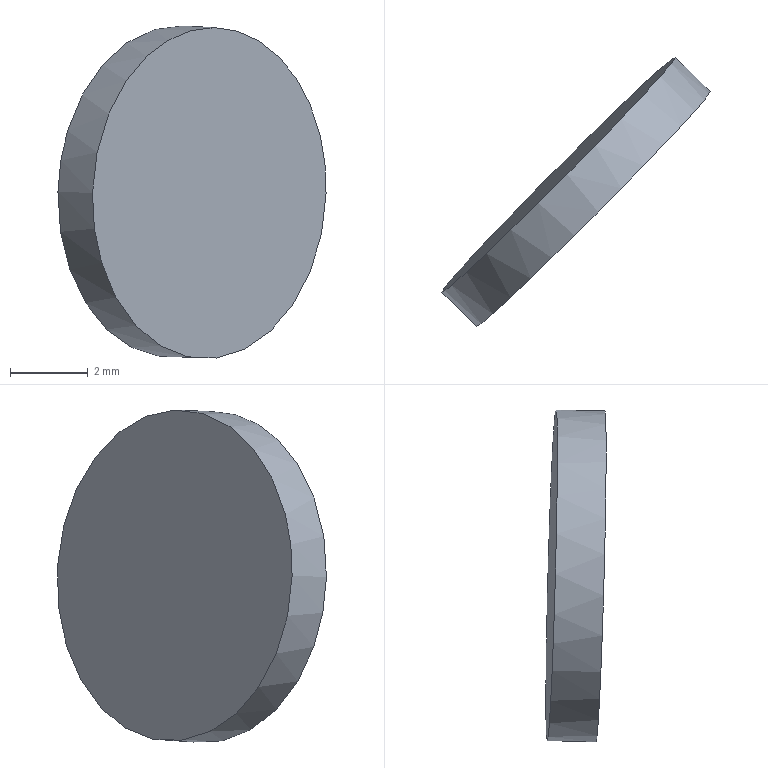Part | STEP file | gslz 2016.10.28-13_id1114_x_t | 1 solid | 3 faces | box 6.882 x 6.913 x 8.538 mm | volume 70.931 mm3 | spline 2 | cylinder 1 | commonest cylinder face diameters 8.5 x1
STEP:
#1=CARTESIAN_POINT('',(0.,0.,0.));
#2=DIRECTION('',(0.,0.,1.));
#3=DIRECTION('',(1.,0.,0.));
#4=AXIS2_PLACEMENT_3D('',#1,#2,#3);
#5=CARTESIAN_POINT('',(428.577,221.709,-30.621));
#6=VERTEX_POINT('',#5);
#7=CARTESIAN_POINT('',(428.577,221.709,-30.621));
#8=CARTESIAN_POINT('',(428.565,221.72,-31.097));
#9=CARTESIAN_POINT('',(428.611,221.79,-31.579));
#10=CARTESIAN_POINT('',(428.711,221.913,-32.027));
#11=CARTESIAN_POINT('',(428.811,222.036,-32.476));
#12=CARTESIAN_POINT('',(428.967,222.214,-32.903));
#13=CARTESIAN_POINT('',(429.168,222.434,-33.275));
#14=CARTESIAN_POINT('',(429.368,222.654,-33.646));
#15=CARTESIAN_POINT('',(429.618,222.921,-33.971));
#16=CARTESIAN_POINT('',(429.896,223.213,-34.223));
#17=CARTESIAN_POINT('',(430.174,223.506,-34.475));
#18=CARTESIAN_POINT('',(430.488,223.831,-34.661));
#19=CARTESIAN_POINT('',(430.813,224.163,-34.765));
#20=CARTESIAN_POINT('',(431.137,224.495,-34.869));
#21=CARTESIAN_POINT('',(431.481,224.842,-34.895));
#22=CARTESIAN_POINT('',(431.815,225.175,-34.84));
#23=CARTESIAN_POINT('',(432.15,225.509,-34.785));
#24=CARTESIAN_POINT('',(432.484,225.839,-34.648));
#25=CARTESIAN_POINT('',(432.791,226.137,-34.44));
#26=CARTESIAN_POINT('',(433.097,226.435,-34.231));
#27=CARTESIAN_POINT('',(433.385,226.71,-33.946));
#28=CARTESIAN_POINT('',(433.629,226.939,-33.608));
#29=CARTESIAN_POINT('',(433.873,227.168,-33.271));
#30=CARTESIAN_POINT('',(434.081,227.357,-32.87));
#31=CARTESIAN_POINT('',(434.235,227.491,-32.441));
#32=CARTESIAN_POINT('',(434.389,227.625,-32.011));
#33=CARTESIAN_POINT('',(434.494,227.708,-31.54));
#34=CARTESIAN_POINT('',(434.541,227.732,-31.068));
#35=CARTESIAN_POINT('',(434.588,227.755,-30.595));
#36=CARTESIAN_POINT('',(434.578,227.721,-30.107));
#37=CARTESIAN_POINT('',(434.512,227.633,-29.644));
#38=CARTESIAN_POINT('',(434.447,227.544,-29.182));
#39=CARTESIAN_POINT('',(434.323,227.397,-28.732));
#40=CARTESIAN_POINT('',(434.152,227.205,-28.331));
#41=CARTESIAN_POINT('',(433.981,227.014,-27.931));
#42=CARTESIAN_POINT('',(433.758,226.771,-27.569));
#43=CARTESIAN_POINT('',(433.502,226.498,-27.276));
#44=CARTESIAN_POINT('',(433.245,226.226,-26.983));
#45=CARTESIAN_POINT('',(432.947,225.915,-26.751));
#46=CARTESIAN_POINT('',(432.633,225.591,-26.598));
#47=CARTESIAN_POINT('',(432.319,225.268,-26.446));
#48=CARTESIAN_POINT('',(431.981,224.924,-26.369));
#49=CARTESIAN_POINT('',(431.645,224.586,-26.374));
#50=CARTESIAN_POINT('',(431.31,224.249,-26.379));
#51=CARTESIAN_POINT('',(430.968,223.91,-26.467));
#52=CARTESIAN_POINT('',(430.649,223.597,-26.629));
#53=CARTESIAN_POINT('',(430.33,223.284,-26.791));
#54=CARTESIAN_POINT('',(430.024,222.988,-27.032));
#55=CARTESIAN_POINT('',(429.757,222.734,-27.333));
#56=CARTESIAN_POINT('',(429.49,222.48,-27.634));
#57=CARTESIAN_POINT('',(429.254,222.261,-28.003));
#58=CARTESIAN_POINT('',(429.07,222.096,-28.409));
#59=CARTESIAN_POINT('',(428.885,221.93,-28.815));
#60=CARTESIAN_POINT('',(428.746,221.813,-29.269));
#61=CARTESIAN_POINT('',(428.665,221.753,-29.734));
#62=CARTESIAN_POINT('',(428.614,221.716,-30.025));
#63=CARTESIAN_POINT('',(428.584,221.701,-30.324));
#64=CARTESIAN_POINT('',(428.577,221.709,-30.621));
#65=B_SPLINE_CURVE_WITH_KNOTS('',3,(#7,#8,#9,#10,#11,#12,#13,#14,#15,#16,#17,#18,#19,#20,#21,#22,#23,#24,#25,#26,#27,#28,#29,#30,#31,#32,#33,#34,#35,#36,#37,#38,#39,#40,#41,#42,#43,#44,#45,#46,#47,#48,#49,#50,#51,#52,#53,#54,#55,#56,#57,#58,#59,#60,#61,#62,#63,#64),.UNSPECIFIED.,.T.,.F.,(1,3,3,3,3,3,3,3,3,3,3,3,3,3,3,3,3,3,3,3,3,1),(-0.03332,0.,0.0537,0.1074,0.1611,0.2148,0.2685,0.3222,0.3759,0.4296,0.4833,0.537,0.5907,0.6445,0.6982,0.7519,0.8056,0.8593,0.913,0.9667,1.,1.054),.UNSPECIFIED.);
#66=CARTESIAN_POINT('',(417.862,211.656,-45.368));
#67=CARTESIAN_POINT('',(417.657,211.178,-39.851));
#68=CARTESIAN_POINT('',(417.452,210.7,-34.333));
#69=CARTESIAN_POINT('',(417.248,210.222,-28.816));
#70=CARTESIAN_POINT('',(417.043,209.744,-23.299));
#71=CARTESIAN_POINT('',(416.839,209.265,-17.782));
#72=CARTESIAN_POINT('',(423.082,216.876,-44.722));
#73=CARTESIAN_POINT('',(422.877,216.398,-39.205));
#74=CARTESIAN_POINT('',(422.673,215.92,-33.688));
#75=CARTESIAN_POINT('',(422.468,215.442,-28.17));
#76=CARTESIAN_POINT('',(422.264,214.964,-22.653));
#77=CARTESIAN_POINT('',(422.059,214.486,-17.136));
#78=CARTESIAN_POINT('',(428.302,222.096,-44.076));
#79=CARTESIAN_POINT('',(428.098,221.618,-38.559));
#80=CARTESIAN_POINT('',(427.893,221.14,-33.042));
#81=CARTESIAN_POINT('',(427.688,220.662,-27.524));
#82=CARTESIAN_POINT('',(427.484,220.184,-22.007));
#83=CARTESIAN_POINT('',(427.279,219.706,-16.49));
#84=CARTESIAN_POINT('',(433.522,227.317,-43.43));
#85=CARTESIAN_POINT('',(433.318,226.839,-37.913));
#86=CARTESIAN_POINT('',(433.113,226.361,-32.396));
#87=CARTESIAN_POINT('',(432.909,225.882,-26.879));
#88=CARTESIAN_POINT('',(432.704,225.404,-21.361));
#89=CARTESIAN_POINT('',(432.5,224.926,-15.844));
#90=CARTESIAN_POINT('',(438.743,232.537,-42.784));
#91=CARTESIAN_POINT('',(438.538,232.059,-37.267));
#92=CARTESIAN_POINT('',(438.334,231.581,-31.75));
#93=CARTESIAN_POINT('',(438.129,231.103,-26.233));
#94=CARTESIAN_POINT('',(437.924,230.625,-20.715));
#95=CARTESIAN_POINT('',(437.72,230.147,-15.198));
#96=CARTESIAN_POINT('',(443.963,237.757,-42.139));
#97=CARTESIAN_POINT('',(443.758,237.279,-36.621));
#98=CARTESIAN_POINT('',(443.554,236.801,-31.104));
#99=CARTESIAN_POINT('',(443.349,236.323,-25.587));
#100=CARTESIAN_POINT('',(443.145,235.845,-20.07));
#101=CARTESIAN_POINT('',(442.94,235.367,-14.552));
#102=B_SPLINE_SURFACE_WITH_KNOTS('',5,5,((#66,#67,#68,#69,#70,#71),(#72,#73,#74,#75,#76,#77),(#78,#79,#80,#81,#82,#83),(#84,#85,#86,#87,#88,#89),(#90,#91,#92,#93,#94,#95),(#96,#97,#98,#99,#100,#101)),.UNSPECIFIED.,.F.,.F.,.F.,(6,6),(6,6),(0.,1.),(0.,1.),.PIECEWISE_BEZIER_KNOTS.);
#103=CARTESIAN_POINT('',(0.4295,0.4843));
#104=CARTESIAN_POINT('',(0.4293,0.4807));
#105=CARTESIAN_POINT('',(0.429,0.4734));
#106=CARTESIAN_POINT('',(0.4291,0.4624));
#107=CARTESIAN_POINT('',(0.4299,0.4515));
#108=CARTESIAN_POINT('',(0.4312,0.4406));
#109=CARTESIAN_POINT('',(0.4331,0.43));
#110=CARTESIAN_POINT('',(0.4356,0.4196));
#111=CARTESIAN_POINT('',(0.4386,0.4094));
#112=CARTESIAN_POINT('',(0.4421,0.3995));
#113=CARTESIAN_POINT('',(0.4462,0.39));
#114=CARTESIAN_POINT('',(0.4508,0.3809));
#115=CARTESIAN_POINT('',(0.4558,0.3723));
#116=CARTESIAN_POINT('',(0.4613,0.3641));
#117=CARTESIAN_POINT('',(0.4672,0.3565));
#118=CARTESIAN_POINT('',(0.4735,0.3495));
#119=CARTESIAN_POINT('',(0.4801,0.3431));
#120=CARTESIAN_POINT('',(0.4871,0.3374));
#121=CARTESIAN_POINT('',(0.4944,0.3323));
#122=CARTESIAN_POINT('',(0.5019,0.328));
#123=CARTESIAN_POINT('',(0.5096,0.3243));
#124=CARTESIAN_POINT('',(0.5175,0.3215));
#125=CARTESIAN_POINT('',(0.5256,0.3194));
#126=CARTESIAN_POINT('',(0.5337,0.318));
#127=CARTESIAN_POINT('',(0.5419,0.3174));
#128=CARTESIAN_POINT('',(0.5501,0.3176));
#129=CARTESIAN_POINT('',(0.5582,0.3186));
#130=CARTESIAN_POINT('',(0.5663,0.3204));
#131=CARTESIAN_POINT('',(0.5743,0.3229));
#132=CARTESIAN_POINT('',(0.5821,0.3262));
#133=CARTESIAN_POINT('',(0.5897,0.3302));
#134=CARTESIAN_POINT('',(0.5971,0.335));
#135=CARTESIAN_POINT('',(0.6042,0.3404));
#136=CARTESIAN_POINT('',(0.6111,0.3466));
#137=CARTESIAN_POINT('',(0.6175,0.3533));
#138=CARTESIAN_POINT('',(0.6236,0.3606));
#139=CARTESIAN_POINT('',(0.6293,0.3685));
#140=CARTESIAN_POINT('',(0.6345,0.3769));
#141=CARTESIAN_POINT('',(0.6393,0.3858));
#142=CARTESIAN_POINT('',(0.6436,0.3951));
#143=CARTESIAN_POINT('',(0.6474,0.4048));
#144=CARTESIAN_POINT('',(0.6506,0.4149));
#145=CARTESIAN_POINT('',(0.6533,0.4253));
#146=CARTESIAN_POINT('',(0.6555,0.4358));
#147=CARTESIAN_POINT('',(0.6571,0.4465));
#148=CARTESIAN_POINT('',(0.6581,0.4574));
#149=CARTESIAN_POINT('',(0.6585,0.4684));
#150=CARTESIAN_POINT('',(0.6584,0.4794));
#151=CARTESIAN_POINT('',(0.6576,0.4903));
#152=CARTESIAN_POINT('',(0.6563,0.501));
#153=CARTESIAN_POINT('',(0.6544,0.5117));
#154=CARTESIAN_POINT('',(0.652,0.5222));
#155=CARTESIAN_POINT('',(0.6489,0.5324));
#156=CARTESIAN_POINT('',(0.6454,0.5422));
#157=CARTESIAN_POINT('',(0.6414,0.5517));
#158=CARTESIAN_POINT('',(0.6368,0.5608));
#159=CARTESIAN_POINT('',(0.6317,0.5695));
#160=CARTESIAN_POINT('',(0.6263,0.5777));
#161=CARTESIAN_POINT('',(0.6204,0.5852));
#162=CARTESIAN_POINT('',(0.6141,0.5922));
#163=CARTESIAN_POINT('',(0.6074,0.5986));
#164=CARTESIAN_POINT('',(0.6004,0.6044));
#165=CARTESIAN_POINT('',(0.5932,0.6095));
#166=CARTESIAN_POINT('',(0.5857,0.6138));
#167=CARTESIAN_POINT('',(0.578,0.6174));
#168=CARTESIAN_POINT('',(0.57,0.6203));
#169=CARTESIAN_POINT('',(0.562,0.6225));
#170=CARTESIAN_POINT('',(0.5539,0.6238));
#171=CARTESIAN_POINT('',(0.5457,0.6244));
#172=CARTESIAN_POINT('',(0.5375,0.6242));
#173=CARTESIAN_POINT('',(0.5293,0.6232));
#174=CARTESIAN_POINT('',(0.5212,0.6214));
#175=CARTESIAN_POINT('',(0.5133,0.6189));
#176=CARTESIAN_POINT('',(0.5055,0.6156));
#177=CARTESIAN_POINT('',(0.4979,0.6116));
#178=CARTESIAN_POINT('',(0.4904,0.6069));
#179=CARTESIAN_POINT('',(0.4833,0.6014));
#180=CARTESIAN_POINT('',(0.4765,0.5954));
#181=CARTESIAN_POINT('',(0.4701,0.5886));
#182=CARTESIAN_POINT('',(0.464,0.5813));
#183=CARTESIAN_POINT('',(0.4583,0.5734));
#184=CARTESIAN_POINT('',(0.453,0.565));
#185=CARTESIAN_POINT('',(0.4483,0.5561));
#186=CARTESIAN_POINT('',(0.444,0.5468));
#187=CARTESIAN_POINT('',(0.4402,0.537));
#188=CARTESIAN_POINT('',(0.4369,0.527));
#189=CARTESIAN_POINT('',(0.4342,0.5167));
#190=CARTESIAN_POINT('',(0.432,0.506));
#191=CARTESIAN_POINT('',(0.4304,0.4952));
#192=CARTESIAN_POINT('',(0.4297,0.4879));
#193=CARTESIAN_POINT('',(0.4295,0.4843));
#194=B_SPLINE_CURVE_WITH_KNOTS('',3,(#103,#104,#105,#106,#107,#108,#109,#110,#111,#112,#113,#114,#115,#116,#117,#118,#119,#120,#121,#122,#123,#124,#125,#126,#127,#128,#129,#130,#131,#132,#133,#134,#135,#136,#137,#138,#139,#140,#141,#142,#143,#144,#145,#146,#147,#148,#149,#150,#151,#152,#153,#154,#155,#156,#157,#158,#159,#160,#161,#162,#163,#164,#165,#166,#167,#168,#169,#170,#171,#172,#173,#174,#175,#176,#177,#178,#179,#180,#181,#182,#183,#184,#185,#186,#187,#188,#189,#190,#191,#192,#193),.UNSPECIFIED.,.T.,.F.,(4,1,1,1,1,1,1,1,1,1,1,1,1,1,1,1,1,1,1,1,1,1,1,1,1,1,1,1,1,1,1,1,1,1,1,1,1,1,1,1,1,1,1,1,1,1,1,1,1,1,1,1,1,1,1,1,1,1,1,1,1,1,1,1,1,1,1,1,1,1,1,1,1,1,1,1,1,1,1,1,1,1,1,1,1,1,1,1,4),(0.,0.01136,0.02273,0.03409,0.04545,0.05682,0.06818,0.07955,0.09091,0.1023,0.1136,0.125,0.1364,0.1477,0.1591,0.1705,0.1818,0.1932,0.2045,0.2159,0.2273,0.2386,0.25,0.2614,0.2727,0.2841,0.2955,0.3068,0.3182,0.3295,0.3409,0.3523,0.3636,0.375,0.3864,0.3977,0.4091,0.4205,0.4318,0.4432,0.4545,0.4659,0.4773,0.4886,0.5,0.5114,0.5227,0.5341,0.5455,0.5568,0.5682,0.5795,0.5909,0.6023,0.6136,0.625,0.6364,0.6477,0.6591,0.6705,0.6818,0.6932,0.7045,0.7159,0.7273,0.7386,0.75,0.7614,0.7727,0.7841,0.7955,0.8068,0.8182,0.8295,0.8409,0.8523,0.8636,0.875,0.8864,0.8977,0.9091,0.9205,0.9318,0.9432,0.9545,0.9659,0.9773,0.9886,1.),.QUASI_UNIFORM_KNOTS.);
#195=(GEOMETRIC_REPRESENTATION_CONTEXT(2)PARAMETRIC_REPRESENTATION_CONTEXT()REPRESENTATION_CONTEXT('',''));
#196=DEFINITIONAL_REPRESENTATION('',(#194),#195);
#197=PCURVE('',#102,#196);
#198=CARTESIAN_POINT('',(433.912,222.398,-30.736));
#199=DIRECTION('',(-0.7088,0.7045,0.03477));
#200=DIRECTION('',(-0.705,-0.7093,0.));
#201=AXIS2_PLACEMENT_3D('',#198,#199,#200);
#202=CYLINDRICAL_SURFACE('',#201,4.25);
#203=CARTESIAN_POINT('',(6.283,3.3));
#204=CARTESIAN_POINT('',(0.,3.3));
#205=B_SPLINE_CURVE_WITH_KNOTS('',1,(#203,#204),.UNSPECIFIED.,.F.,.F.,(2,2),(0.,1.),.PIECEWISE_BEZIER_KNOTS.);
#206=(GEOMETRIC_REPRESENTATION_CONTEXT(2)PARAMETRIC_REPRESENTATION_CONTEXT()REPRESENTATION_CONTEXT('',''));
#207=DEFINITIONAL_REPRESENTATION('',(#205),#206);
#208=PCURVE('',#202,#207);
#209=SURFACE_CURVE('',#65,(#197,#208),.PCURVE_S1.);
#210=EDGE_CURVE('',#6,#6,#209,.T.);
#211=ORIENTED_EDGE('',*,*,#210,.T.);
#212=EDGE_LOOP('',(#211));
#213=FACE_BOUND('',#212,.F.);
#214=ADVANCED_FACE('',(#213),#102,.F.);
#215=CARTESIAN_POINT('',(435.455,226.857,-30.665));
#216=VERTEX_POINT('',#215);
#217=CARTESIAN_POINT('',(429.463,220.828,-30.665));
#218=VERTEX_POINT('',#217);
#219=CARTESIAN_POINT('',(435.455,226.857,-30.665));
#220=CARTESIAN_POINT('',(435.443,226.868,-31.14));
#221=CARTESIAN_POINT('',(435.373,226.822,-31.622));
#222=CARTESIAN_POINT('',(435.251,226.721,-32.071));
#223=CARTESIAN_POINT('',(435.129,226.621,-32.519));
#224=CARTESIAN_POINT('',(434.951,226.463,-32.947));
#225=CARTESIAN_POINT('',(434.733,226.261,-33.318));
#226=CARTESIAN_POINT('',(434.514,226.06,-33.689));
#227=CARTESIAN_POINT('',(434.249,225.808,-34.014));
#228=CARTESIAN_POINT('',(433.958,225.528,-34.266));
#229=CARTESIAN_POINT('',(433.667,225.249,-34.518));
#230=CARTESIAN_POINT('',(433.344,224.932,-34.704));
#231=CARTESIAN_POINT('',(433.014,224.606,-34.809));
#232=CARTESIAN_POINT('',(432.684,224.279,-34.913));
#233=CARTESIAN_POINT('',(432.339,223.933,-34.939));
#234=CARTESIAN_POINT('',(432.008,223.597,-34.884));
#235=CARTESIAN_POINT('',(431.676,223.26,-34.829));
#236=CARTESIAN_POINT('',(431.348,222.924,-34.691));
#237=CARTESIAN_POINT('',(431.052,222.616,-34.483));
#238=CARTESIAN_POINT('',(430.756,222.307,-34.275));
#239=CARTESIAN_POINT('',(430.483,222.018,-33.99));
#240=CARTESIAN_POINT('',(430.255,221.773,-33.652));
#241=CARTESIAN_POINT('',(430.028,221.527,-33.314));
#242=CARTESIAN_POINT('',(429.84,221.318,-32.914));
#243=CARTESIAN_POINT('',(429.707,221.163,-32.484));
#244=CARTESIAN_POINT('',(429.573,221.008,-32.054));
#245=CARTESIAN_POINT('',(429.492,220.903,-31.584));
#246=CARTESIAN_POINT('',(429.468,220.856,-31.111));
#247=CARTESIAN_POINT('',(429.445,220.809,-30.638));
#248=CARTESIAN_POINT('',(429.479,220.819,-30.15));
#249=CARTESIAN_POINT('',(429.567,220.885,-29.688));
#250=CARTESIAN_POINT('',(429.656,220.951,-29.225));
#251=CARTESIAN_POINT('',(429.801,221.075,-28.775));
#252=CARTESIAN_POINT('',(429.992,221.247,-28.375));
#253=CARTESIAN_POINT('',(430.183,221.42,-27.974));
#254=CARTESIAN_POINT('',(430.424,221.644,-27.613));
#255=CARTESIAN_POINT('',(430.695,221.903,-27.32));
#256=CARTESIAN_POINT('',(430.966,222.161,-27.027));
#257=CARTESIAN_POINT('',(431.275,222.461,-26.794));
#258=CARTESIAN_POINT('',(431.597,222.777,-26.642));
#259=CARTESIAN_POINT('',(431.918,223.092,-26.489));
#260=CARTESIAN_POINT('',(432.261,223.433,-26.412));
#261=CARTESIAN_POINT('',(432.596,223.771,-26.418));
#262=CARTESIAN_POINT('',(432.931,224.108,-26.423));
#263=CARTESIAN_POINT('',(433.268,224.452,-26.51));
#264=CARTESIAN_POINT('',(433.579,224.773,-26.672));
#265=CARTESIAN_POINT('',(433.891,225.094,-26.834));
#266=CARTESIAN_POINT('',(434.184,225.401,-27.076));
#267=CARTESIAN_POINT('',(434.437,225.67,-27.377));
#268=CARTESIAN_POINT('',(434.689,225.938,-27.678));
#269=CARTESIAN_POINT('',(434.906,226.175,-28.046));
#270=CARTESIAN_POINT('',(435.071,226.361,-28.452));
#271=CARTESIAN_POINT('',(435.235,226.547,-28.858));
#272=CARTESIAN_POINT('',(435.352,226.686,-29.312));
#273=CARTESIAN_POINT('',(435.41,226.768,-29.777));
#274=CARTESIAN_POINT('',(435.447,226.82,-30.068));
#275=CARTESIAN_POINT('',(435.462,226.849,-30.367));
#276=CARTESIAN_POINT('',(435.455,226.857,-30.665));
#277=B_SPLINE_CURVE_WITH_KNOTS('',3,(#219,#220,#221,#222,#223,#224,#225,#226,#227,#228,#229,#230,#231,#232,#233,#234,#235,#236,#237,#238,#239,#240,#241,#242,#243,#244,#245,#246,#247,#248,#249,#250,#251,#252,#253,#254,#255,#256,#257,#258,#259,#260,#261,#262,#263,#264,#265,#266,#267,#268,#269,#270,#271,#272,#273,#274,#275,#276),.UNSPECIFIED.,.T.,.F.,(1,3,3,3,3,3,3,3,3,3,3,3,3,3,3,3,3,3,3,3,3,1),(-0.03332,0.,0.0537,0.1074,0.1611,0.2148,0.2685,0.3222,0.3759,0.4296,0.4833,0.537,0.5907,0.6445,0.6982,0.7519,0.8056,0.8593,0.913,0.9667,1.,1.054),.UNSPECIFIED.);
#278=CARTESIAN_POINT('',(3.142,2.05));
#279=CARTESIAN_POINT('',(9.425,2.05));
#280=B_SPLINE_CURVE_WITH_KNOTS('',1,(#278,#279),.UNSPECIFIED.,.F.,.F.,(2,2),(0.,1.),.PIECEWISE_BEZIER_KNOTS.);
#281=(GEOMETRIC_REPRESENTATION_CONTEXT(2)PARAMETRIC_REPRESENTATION_CONTEXT()REPRESENTATION_CONTEXT('',''));
#282=DEFINITIONAL_REPRESENTATION('',(#280),#281);
#283=PCURVE('',#202,#282);
#284=CARTESIAN_POINT('',(429.583,221.18,-35.348));
#285=CARTESIAN_POINT('',(429.477,220.931,-32.476));
#286=CARTESIAN_POINT('',(429.37,220.683,-29.604));
#287=CARTESIAN_POINT('',(429.264,220.434,-26.732));
#288=CARTESIAN_POINT('',(431.607,223.204,-35.098));
#289=CARTESIAN_POINT('',(431.501,222.955,-32.226));
#290=CARTESIAN_POINT('',(431.394,222.707,-29.354));
#291=CARTESIAN_POINT('',(431.288,222.458,-26.482));
#292=CARTESIAN_POINT('',(433.631,225.228,-34.847));
#293=CARTESIAN_POINT('',(433.525,224.979,-31.975));
#294=CARTESIAN_POINT('',(433.418,224.731,-29.103));
#295=CARTESIAN_POINT('',(433.312,224.482,-26.231));
#296=CARTESIAN_POINT('',(435.655,227.252,-34.597));
#297=CARTESIAN_POINT('',(435.549,227.003,-31.725));
#298=CARTESIAN_POINT('',(435.442,226.754,-28.853));
#299=CARTESIAN_POINT('',(435.336,226.506,-25.981));
#300=B_SPLINE_SURFACE_WITH_KNOTS('',3,3,((#284,#285,#286,#287),(#288,#289,#290,#291),(#292,#293,#294,#295),(#296,#297,#298,#299)),.UNSPECIFIED.,.F.,.F.,.F.,(4,4),(4,4),(0.,1.),(0.,1.),.PIECEWISE_BEZIER_KNOTS.);
#301=CARTESIAN_POINT('',(0.9911,0.4571));
#302=CARTESIAN_POINT('',(0.99,0.4455));
#303=CARTESIAN_POINT('',(0.9871,0.4224));
#304=CARTESIAN_POINT('',(0.9803,0.3879));
#305=CARTESIAN_POINT('',(0.971,0.354));
#306=CARTESIAN_POINT('',(0.9594,0.3208));
#307=CARTESIAN_POINT('',(0.9455,0.2888));
#308=CARTESIAN_POINT('',(0.9292,0.2577));
#309=CARTESIAN_POINT('',(0.9107,0.2278));
#310=CARTESIAN_POINT('',(0.8901,0.1992));
#311=CARTESIAN_POINT('',(0.8676,0.1722));
#312=CARTESIAN_POINT('',(0.8433,0.147));
#313=CARTESIAN_POINT('',(0.8172,0.1236));
#314=CARTESIAN_POINT('',(0.7893,0.1019));
#315=CARTESIAN_POINT('',(0.76,0.08232));
#316=CARTESIAN_POINT('',(0.7295,0.0649));
#317=CARTESIAN_POINT('',(0.6979,0.04978));
#318=CARTESIAN_POINT('',(0.6651,0.03686));
#319=CARTESIAN_POINT('',(0.6314,0.02629));
#320=CARTESIAN_POINT('',(0.5971,0.0181));
#321=CARTESIAN_POINT('',(0.5625,0.01242));
#322=CARTESIAN_POINT('',(0.5275,0.009248));
#323=CARTESIAN_POINT('',(0.4922,0.008564));
#324=CARTESIAN_POINT('',(0.4569,0.01036));
#325=CARTESIAN_POINT('',(0.422,0.01463));
#326=CARTESIAN_POINT('',(0.3876,0.02135));
#327=CARTESIAN_POINT('',(0.3536,0.03058));
#328=CARTESIAN_POINT('',(0.3203,0.04222));
#329=CARTESIAN_POINT('',(0.2879,0.05616));
#330=CARTESIAN_POINT('',(0.2566,0.07232));
#331=CARTESIAN_POINT('',(0.2268,0.0906));
#332=CARTESIAN_POINT('',(0.1982,0.1111));
#333=CARTESIAN_POINT('',(0.171,0.1336));
#334=CARTESIAN_POINT('',(0.1455,0.1579));
#335=CARTESIAN_POINT('',(0.122,0.1839));
#336=CARTESIAN_POINT('',(0.1004,0.2114));
#337=CARTESIAN_POINT('',(0.08075,0.2406));
#338=CARTESIAN_POINT('',(0.06321,0.2711));
#339=CARTESIAN_POINT('',(0.04788,0.3028));
#340=CARTESIAN_POINT('',(0.03495,0.3353));
#341=CARTESIAN_POINT('',(0.02438,0.3687));
#342=CARTESIAN_POINT('',(0.0162,0.4029));
#343=CARTESIAN_POINT('',(0.01046,0.4376));
#344=CARTESIAN_POINT('',(0.007195,0.4725));
#345=CARTESIAN_POINT('',(0.006481,0.5074));
#346=CARTESIAN_POINT('',(0.007694,0.5307));
#347=CARTESIAN_POINT('',(0.008723,0.5424));
#348=B_SPLINE_CURVE_WITH_KNOTS('',3,(#301,#302,#303,#304,#305,#306,#307,#308,#309,#310,#311,#312,#313,#314,#315,#316,#317,#318,#319,#320,#321,#322,#323,#324,#325,#326,#327,#328,#329,#330,#331,#332,#333,#334,#335,#336,#337,#338,#339,#340,#341,#342,#343,#344,#345,#346,#347),.UNSPECIFIED.,.F.,.F.,(4,1,1,1,1,1,1,1,1,1,1,1,1,1,1,1,1,1,1,1,1,1,1,1,1,1,1,1,1,1,1,1,1,1,1,1,1,1,1,1,1,1,1,1,4),(0.,0.01136,0.02273,0.03409,0.04545,0.05682,0.06818,0.07955,0.09091,0.1023,0.1136,0.125,0.1364,0.1477,0.1591,0.1705,0.1818,0.1932,0.2045,0.2159,0.2273,0.2386,0.25,0.2614,0.2727,0.2841,0.2955,0.3068,0.3182,0.3295,0.3409,0.3523,0.3636,0.375,0.3864,0.3977,0.4091,0.4205,0.4318,0.4432,0.4545,0.4659,0.4773,0.4886,0.5),.QUASI_UNIFORM_KNOTS.);
#349=(GEOMETRIC_REPRESENTATION_CONTEXT(2)PARAMETRIC_REPRESENTATION_CONTEXT()REPRESENTATION_CONTEXT('',''));
#350=DEFINITIONAL_REPRESENTATION('',(#348),#349);
#351=PCURVE('',#300,#350);
#352=SURFACE_CURVE('',#277,(#283,#351),.PCURVE_S1.);
#353=EDGE_CURVE('',#216,#218,#352,.T.);
#354=ORIENTED_EDGE('',*,*,#353,.T.);
#355=CARTESIAN_POINT('',(429.463,220.828,-30.665));
#356=CARTESIAN_POINT('',(428.577,221.709,-30.621));
#357=B_SPLINE_CURVE_WITH_KNOTS('',1,(#355,#356),.UNSPECIFIED.,.F.,.F.,(2,2),(2.05,3.3),.PIECEWISE_BEZIER_KNOTS.);
#358=CARTESIAN_POINT('',(6.283,0.));
#359=DIRECTION('',(0.,1.));
#360=VECTOR('',#359,1.);
#361=LINE('',#358,#360);
#362=(GEOMETRIC_REPRESENTATION_CONTEXT(2)PARAMETRIC_REPRESENTATION_CONTEXT()REPRESENTATION_CONTEXT('',''));
#363=DEFINITIONAL_REPRESENTATION('',(#361),#362);
#364=PCURVE('',#202,#363);
#365=CARTESIAN_POINT('',(0.,0.));
#366=DIRECTION('',(0.,1.));
#367=VECTOR('',#366,1.);
#368=LINE('',#365,#367);
#369=(GEOMETRIC_REPRESENTATION_CONTEXT(2)PARAMETRIC_REPRESENTATION_CONTEXT()REPRESENTATION_CONTEXT('',''));
#370=DEFINITIONAL_REPRESENTATION('',(#368),#369);
#371=PCURVE('',#202,#370);
#372=SEAM_CURVE('',#357,(#364,#371),.PCURVE_S1.);
#373=EDGE_CURVE('',#218,#6,#372,.T.);
#374=ORIENTED_EDGE('',*,*,#373,.T.);
#375=ORIENTED_EDGE('',*,*,#210,.T.);
#376=ORIENTED_EDGE('',*,*,#373,.F.);
#377=CARTESIAN_POINT('',(435.455,226.857,-30.665));
#378=CARTESIAN_POINT('',(435.443,226.868,-31.14));
#379=CARTESIAN_POINT('',(435.373,226.822,-31.622));
#380=CARTESIAN_POINT('',(435.251,226.721,-32.071));
#381=CARTESIAN_POINT('',(435.129,226.621,-32.519));
#382=CARTESIAN_POINT('',(434.951,226.463,-32.947));
#383=CARTESIAN_POINT('',(434.733,226.261,-33.318));
#384=CARTESIAN_POINT('',(434.514,226.06,-33.689));
#385=CARTESIAN_POINT('',(434.249,225.808,-34.014));
#386=CARTESIAN_POINT('',(433.958,225.528,-34.266));
#387=CARTESIAN_POINT('',(433.667,225.249,-34.518));
#388=CARTESIAN_POINT('',(433.344,224.932,-34.704));
#389=CARTESIAN_POINT('',(433.014,224.606,-34.809));
#390=CARTESIAN_POINT('',(432.684,224.279,-34.913));
#391=CARTESIAN_POINT('',(432.339,223.933,-34.939));
#392=CARTESIAN_POINT('',(432.008,223.597,-34.884));
#393=CARTESIAN_POINT('',(431.676,223.26,-34.829));
#394=CARTESIAN_POINT('',(431.348,222.924,-34.691));
#395=CARTESIAN_POINT('',(431.052,222.616,-34.483));
#396=CARTESIAN_POINT('',(430.756,222.307,-34.275));
#397=CARTESIAN_POINT('',(430.483,222.018,-33.99));
#398=CARTESIAN_POINT('',(430.255,221.773,-33.652));
#399=CARTESIAN_POINT('',(430.028,221.527,-33.314));
#400=CARTESIAN_POINT('',(429.84,221.318,-32.914));
#401=CARTESIAN_POINT('',(429.707,221.163,-32.484));
#402=CARTESIAN_POINT('',(429.573,221.008,-32.054));
#403=CARTESIAN_POINT('',(429.492,220.903,-31.584));
#404=CARTESIAN_POINT('',(429.468,220.856,-31.111));
#405=CARTESIAN_POINT('',(429.445,220.809,-30.638));
#406=CARTESIAN_POINT('',(429.479,220.819,-30.15));
#407=CARTESIAN_POINT('',(429.567,220.885,-29.688));
#408=CARTESIAN_POINT('',(429.656,220.951,-29.225));
#409=CARTESIAN_POINT('',(429.801,221.075,-28.775));
#410=CARTESIAN_POINT('',(429.992,221.247,-28.375));
#411=CARTESIAN_POINT('',(430.183,221.42,-27.974));
#412=CARTESIAN_POINT('',(430.424,221.644,-27.613));
#413=CARTESIAN_POINT('',(430.695,221.903,-27.32));
#414=CARTESIAN_POINT('',(430.966,222.161,-27.027));
#415=CARTESIAN_POINT('',(431.275,222.461,-26.794));
#416=CARTESIAN_POINT('',(431.597,222.777,-26.642));
#417=CARTESIAN_POINT('',(431.918,223.092,-26.489));
#418=CARTESIAN_POINT('',(432.261,223.433,-26.412));
#419=CARTESIAN_POINT('',(432.596,223.771,-26.418));
#420=CARTESIAN_POINT('',(432.931,224.108,-26.423));
#421=CARTESIAN_POINT('',(433.268,224.452,-26.51));
#422=CARTESIAN_POINT('',(433.579,224.773,-26.672));
#423=CARTESIAN_POINT('',(433.891,225.094,-26.834));
#424=CARTESIAN_POINT('',(434.184,225.401,-27.076));
#425=CARTESIAN_POINT('',(434.437,225.67,-27.377));
#426=CARTESIAN_POINT('',(434.689,225.938,-27.678));
#427=CARTESIAN_POINT('',(434.906,226.175,-28.046));
#428=CARTESIAN_POINT('',(435.071,226.361,-28.452));
#429=CARTESIAN_POINT('',(435.235,226.547,-28.858));
#430=CARTESIAN_POINT('',(435.352,226.686,-29.312));
#431=CARTESIAN_POINT('',(435.41,226.768,-29.777));
#432=CARTESIAN_POINT('',(435.447,226.82,-30.068));
#433=CARTESIAN_POINT('',(435.462,226.849,-30.367));
#434=CARTESIAN_POINT('',(435.455,226.857,-30.665));
#435=B_SPLINE_CURVE_WITH_KNOTS('',3,(#377,#378,#379,#380,#381,#382,#383,#384,#385,#386,#387,#388,#389,#390,#391,#392,#393,#394,#395,#396,#397,#398,#399,#400,#401,#402,#403,#404,#405,#406,#407,#408,#409,#410,#411,#412,#413,#414,#415,#416,#417,#418,#419,#420,#421,#422,#423,#424,#425,#426,#427,#428,#429,#430,#431,#432,#433,#434),.UNSPECIFIED.,.T.,.F.,(1,3,3,3,3,3,3,3,3,3,3,3,3,3,3,3,3,3,3,3,3,1),(-0.03332,0.,0.0537,0.1074,0.1611,0.2148,0.2685,0.3222,0.3759,0.4296,0.4833,0.537,0.5907,0.6445,0.6982,0.7519,0.8056,0.8593,0.913,0.9667,1.,1.054),.UNSPECIFIED.);
#436=CARTESIAN_POINT('',(-3.142,2.05));
#437=CARTESIAN_POINT('',(3.142,2.05));
#438=B_SPLINE_CURVE_WITH_KNOTS('',1,(#436,#437),.UNSPECIFIED.,.F.,.F.,(2,2),(0.,1.),.PIECEWISE_BEZIER_KNOTS.);
#439=(GEOMETRIC_REPRESENTATION_CONTEXT(2)PARAMETRIC_REPRESENTATION_CONTEXT()REPRESENTATION_CONTEXT('',''));
#440=DEFINITIONAL_REPRESENTATION('',(#438),#439);
#441=PCURVE('',#202,#440);
#442=CARTESIAN_POINT('',(0.008723,0.5424));
#443=CARTESIAN_POINT('',(0.009748,0.5541));
#444=CARTESIAN_POINT('',(0.01263,0.5773));
#445=CARTESIAN_POINT('',(0.01941,0.6118));
#446=CARTESIAN_POINT('',(0.0286,0.6457));
#447=CARTESIAN_POINT('',(0.04019,0.6786));
#448=CARTESIAN_POINT('',(0.05421,0.7109));
#449=CARTESIAN_POINT('',(0.07049,0.7421));
#450=CARTESIAN_POINT('',(0.08894,0.772));
#451=CARTESIAN_POINT('',(0.1094,0.8005));
#452=CARTESIAN_POINT('',(0.1318,0.8273));
#453=CARTESIAN_POINT('',(0.1563,0.8527));
#454=CARTESIAN_POINT('',(0.1825,0.8763));
#455=CARTESIAN_POINT('',(0.2103,0.8979));
#456=CARTESIAN_POINT('',(0.2394,0.9174));
#457=CARTESIAN_POINT('',(0.2699,0.9348));
#458=CARTESIAN_POINT('',(0.3017,0.95));
#459=CARTESIAN_POINT('',(0.3345,0.963));
#460=CARTESIAN_POINT('',(0.3681,0.9736));
#461=CARTESIAN_POINT('',(0.4022,0.9817));
#462=CARTESIAN_POINT('',(0.437,0.9874));
#463=CARTESIAN_POINT('',(0.4721,0.9906));
#464=CARTESIAN_POINT('',(0.5074,0.9914));
#465=CARTESIAN_POINT('',(0.5425,0.9896));
#466=CARTESIAN_POINT('',(0.5773,0.9854));
#467=CARTESIAN_POINT('',(0.6119,0.9786));
#468=CARTESIAN_POINT('',(0.646,0.9694));
#469=CARTESIAN_POINT('',(0.6793,0.9578));
#470=CARTESIAN_POINT('',(0.7115,0.944));
#471=CARTESIAN_POINT('',(0.7427,0.9278));
#472=CARTESIAN_POINT('',(0.7728,0.9094));
#473=CARTESIAN_POINT('',(0.8015,0.8889));
#474=CARTESIAN_POINT('',(0.8286,0.8665));
#475=CARTESIAN_POINT('',(0.8539,0.8424));
#476=CARTESIAN_POINT('',(0.8775,0.8163));
#477=CARTESIAN_POINT('',(0.8992,0.7886));
#478=CARTESIAN_POINT('',(0.9189,0.7594));
#479=CARTESIAN_POINT('',(0.9365,0.729));
#480=CARTESIAN_POINT('',(0.9517,0.6976));
#481=CARTESIAN_POINT('',(0.9647,0.6649));
#482=CARTESIAN_POINT('',(0.9753,0.6314));
#483=CARTESIAN_POINT('',(0.9836,0.5972));
#484=CARTESIAN_POINT('',(0.9893,0.5628));
#485=CARTESIAN_POINT('',(0.9926,0.5276));
#486=CARTESIAN_POINT('',(0.9933,0.4923));
#487=CARTESIAN_POINT('',(0.9921,0.4688));
#488=CARTESIAN_POINT('',(0.9911,0.4571));
#489=B_SPLINE_CURVE_WITH_KNOTS('',3,(#442,#443,#444,#445,#446,#447,#448,#449,#450,#451,#452,#453,#454,#455,#456,#457,#458,#459,#460,#461,#462,#463,#464,#465,#466,#467,#468,#469,#470,#471,#472,#473,#474,#475,#476,#477,#478,#479,#480,#481,#482,#483,#484,#485,#486,#487,#488),.UNSPECIFIED.,.F.,.F.,(4,1,1,1,1,1,1,1,1,1,1,1,1,1,1,1,1,1,1,1,1,1,1,1,1,1,1,1,1,1,1,1,1,1,1,1,1,1,1,1,1,1,1,1,4),(0.5,0.5114,0.5227,0.5341,0.5455,0.5568,0.5682,0.5795,0.5909,0.6023,0.6136,0.625,0.6364,0.6477,0.6591,0.6705,0.6818,0.6932,0.7045,0.7159,0.7273,0.7386,0.75,0.7614,0.7727,0.7841,0.7955,0.8068,0.8182,0.8295,0.8409,0.8523,0.8636,0.875,0.8864,0.8977,0.9091,0.9205,0.9318,0.9432,0.9545,0.9659,0.9773,0.9886,1.),.QUASI_UNIFORM_KNOTS.);
#490=(GEOMETRIC_REPRESENTATION_CONTEXT(2)PARAMETRIC_REPRESENTATION_CONTEXT()REPRESENTATION_CONTEXT('',''));
#491=DEFINITIONAL_REPRESENTATION('',(#489),#490);
#492=PCURVE('',#300,#491);
#493=SURFACE_CURVE('',#435,(#441,#492),.PCURVE_S1.);
#494=EDGE_CURVE('',#218,#216,#493,.T.);
#495=ORIENTED_EDGE('',*,*,#494,.T.);
#496=EDGE_LOOP('',(#354,#374,#375,#376,#495));
#497=FACE_BOUND('',#496,.T.);
#498=ADVANCED_FACE('',(#497),#202,.T.);
#499=ORIENTED_EDGE('',*,*,#353,.F.);
#500=ORIENTED_EDGE('',*,*,#494,.F.);
#501=EDGE_LOOP('',(#499,#500));
#502=FACE_BOUND('',#501,.T.);
#503=ADVANCED_FACE('',(#502),#300,.T.);
#504=CLOSED_SHELL('',(#214,#498,#503));
#505=MANIFOLD_SOLID_BREP('',#504);
#506=(LENGTH_UNIT()NAMED_UNIT(*)SI_UNIT(.MILLI.,.METRE.));
#507=UNCERTAINTY_MEASURE_WITH_UNIT(LENGTH_MEASURE(0.005),#506,'','');
#508=(NAMED_UNIT(*)PLANE_ANGLE_UNIT()SI_UNIT($,.RADIAN.));
#509=(NAMED_UNIT(*)SI_UNIT($,.STERADIAN.)SOLID_ANGLE_UNIT());
#510=(GEOMETRIC_REPRESENTATION_CONTEXT(3)GLOBAL_UNCERTAINTY_ASSIGNED_CONTEXT((#507))GLOBAL_UNIT_ASSIGNED_CONTEXT((#506,#508,#509))REPRESENTATION_CONTEXT('',''));
#511=ADVANCED_BREP_SHAPE_REPRESENTATION('',(#4,#505),#510);